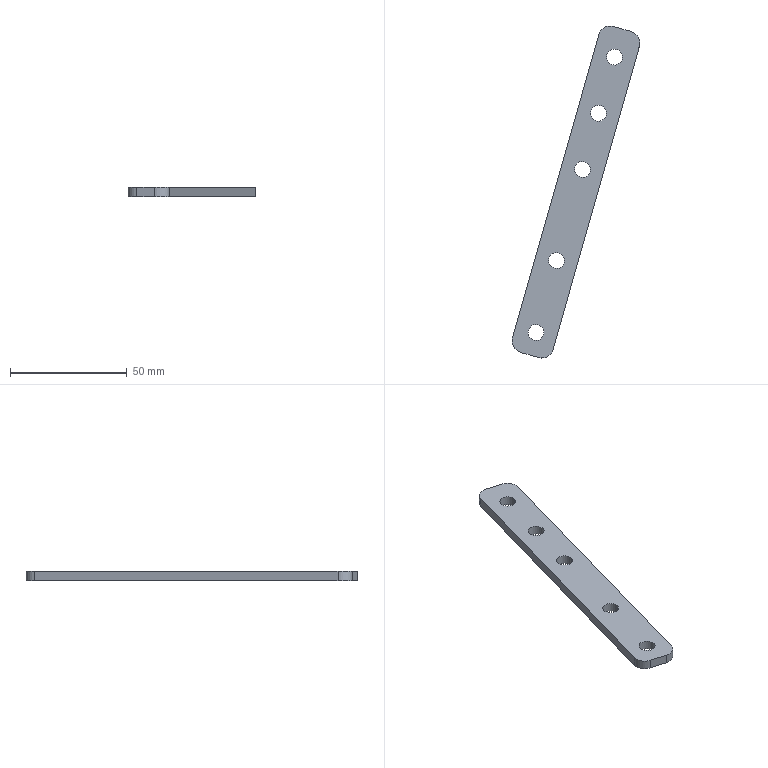Part | SolidWorks | features BaseBody 1 | 1 solid | 20 faces | box 54.655 x 142.032 x 4 mm | volume 9628 mm3 | cylinder 14 | plane 6 | commonest cylinder face diameters 6.8 x10 10 x4
STEP:
#1=CARTESIAN_POINT('',(427.437,245.838,55.5));
#2=VERTEX_POINT('',#1);
#3=CARTESIAN_POINT('',(420.897,247.7,55.5));
#4=VERTEX_POINT('',#3);
#5=CARTESIAN_POINT('',(424.167,246.769,55.5));
#6=DIRECTION('',(0.,0.,1.));
#7=DIRECTION('',(-0.9618,0.2738,0.));
#8=AXIS2_PLACEMENT_3D('',#5,#6,#7);
#9=CIRCLE('',#8,3.4);
#10=EDGE_CURVE('',#2,#4,#9,.T.);
#11=ORIENTED_EDGE('',*,*,#10,.F.);
#12=CARTESIAN_POINT('',(427.437,245.838,59.5));
#13=VERTEX_POINT('',#12);
#14=CARTESIAN_POINT('',(427.437,245.838,59.5));
#15=DIRECTION('',(0.,0.,1.));
#16=VECTOR('',#15,1000.);
#17=LINE('',#14,#16);
#18=EDGE_CURVE('',#2,#13,#17,.T.);
#19=ORIENTED_EDGE('',*,*,#18,.T.);
#20=CARTESIAN_POINT('',(420.897,247.7,59.5));
#21=VERTEX_POINT('',#20);
#22=CARTESIAN_POINT('',(424.167,246.769,59.5));
#23=DIRECTION('',(0.,0.,1.));
#24=DIRECTION('',(-0.9618,0.2738,0.));
#25=AXIS2_PLACEMENT_3D('',#22,#23,#24);
#26=CIRCLE('',#25,3.4);
#27=EDGE_CURVE('',#13,#21,#26,.T.);
#28=ORIENTED_EDGE('',*,*,#27,.T.);
#29=CARTESIAN_POINT('',(420.897,247.7,59.5));
#30=DIRECTION('',(0.,0.,1.));
#31=VECTOR('',#30,1000.);
#32=LINE('',#29,#31);
#33=EDGE_CURVE('',#4,#21,#32,.T.);
#34=ORIENTED_EDGE('',*,*,#33,.F.);
#35=EDGE_LOOP('',(#11,#19,#28,#34));
#36=FACE_OUTER_BOUND('',#35,.T.);
#37=CARTESIAN_POINT('',(424.167,246.769,59.5));
#38=DIRECTION('',(0.,0.,1.));
#39=DIRECTION('',(-0.9618,0.2738,0.));
#40=AXIS2_PLACEMENT_3D('',#37,#38,#39);
#41=CYLINDRICAL_SURFACE('',#40,3.4);
#42=ADVANCED_FACE('',(#36),#41,.F.);
#43=CARTESIAN_POINT('',(420.593,221.793,55.5));
#44=VERTEX_POINT('',#43);
#45=CARTESIAN_POINT('',(414.053,223.655,55.5));
#46=VERTEX_POINT('',#45);
#47=CARTESIAN_POINT('',(417.323,222.724,55.5));
#48=DIRECTION('',(0.,0.,1.));
#49=DIRECTION('',(-0.9618,0.2738,0.));
#50=AXIS2_PLACEMENT_3D('',#47,#48,#49);
#51=CIRCLE('',#50,3.4);
#52=EDGE_CURVE('',#44,#46,#51,.T.);
#53=ORIENTED_EDGE('',*,*,#52,.F.);
#54=CARTESIAN_POINT('',(420.593,221.793,59.5));
#55=VERTEX_POINT('',#54);
#56=CARTESIAN_POINT('',(420.593,221.793,59.5));
#57=DIRECTION('',(0.,0.,1.));
#58=VECTOR('',#57,1000.);
#59=LINE('',#56,#58);
#60=EDGE_CURVE('',#44,#55,#59,.T.);
#61=ORIENTED_EDGE('',*,*,#60,.T.);
#62=CARTESIAN_POINT('',(414.053,223.655,59.5));
#63=VERTEX_POINT('',#62);
#64=CARTESIAN_POINT('',(417.323,222.724,59.5));
#65=DIRECTION('',(0.,0.,1.));
#66=DIRECTION('',(-0.9618,0.2738,0.));
#67=AXIS2_PLACEMENT_3D('',#64,#65,#66);
#68=CIRCLE('',#67,3.4);
#69=EDGE_CURVE('',#55,#63,#68,.T.);
#70=ORIENTED_EDGE('',*,*,#69,.T.);
#71=CARTESIAN_POINT('',(414.053,223.655,59.5));
#72=DIRECTION('',(0.,0.,1.));
#73=VECTOR('',#72,1000.);
#74=LINE('',#71,#73);
#75=EDGE_CURVE('',#46,#63,#74,.T.);
#76=ORIENTED_EDGE('',*,*,#75,.F.);
#77=EDGE_LOOP('',(#53,#61,#70,#76));
#78=FACE_OUTER_BOUND('',#77,.T.);
#79=CARTESIAN_POINT('',(417.323,222.724,59.5));
#80=DIRECTION('',(0.,0.,1.));
#81=DIRECTION('',(-0.9618,0.2738,0.));
#82=AXIS2_PLACEMENT_3D('',#79,#80,#81);
#83=CYLINDRICAL_SURFACE('',#82,3.4);
#84=ADVANCED_FACE('',(#78),#83,.F.);
#85=CARTESIAN_POINT('',(413.748,197.748,55.5));
#86=VERTEX_POINT('',#85);
#87=CARTESIAN_POINT('',(407.208,199.61,55.5));
#88=VERTEX_POINT('',#87);
#89=CARTESIAN_POINT('',(410.478,198.679,55.5));
#90=DIRECTION('',(0.,0.,1.));
#91=DIRECTION('',(-0.9618,0.2738,0.));
#92=AXIS2_PLACEMENT_3D('',#89,#90,#91);
#93=CIRCLE('',#92,3.4);
#94=EDGE_CURVE('',#86,#88,#93,.T.);
#95=ORIENTED_EDGE('',*,*,#94,.F.);
#96=CARTESIAN_POINT('',(413.748,197.748,59.5));
#97=VERTEX_POINT('',#96);
#98=CARTESIAN_POINT('',(413.748,197.748,59.5));
#99=DIRECTION('',(0.,0.,1.));
#100=VECTOR('',#99,1000.);
#101=LINE('',#98,#100);
#102=EDGE_CURVE('',#86,#97,#101,.T.);
#103=ORIENTED_EDGE('',*,*,#102,.T.);
#104=CARTESIAN_POINT('',(407.208,199.61,59.5));
#105=VERTEX_POINT('',#104);
#106=CARTESIAN_POINT('',(410.478,198.679,59.5));
#107=DIRECTION('',(0.,0.,1.));
#108=DIRECTION('',(-0.9618,0.2738,0.));
#109=AXIS2_PLACEMENT_3D('',#106,#107,#108);
#110=CIRCLE('',#109,3.4);
#111=EDGE_CURVE('',#97,#105,#110,.T.);
#112=ORIENTED_EDGE('',*,*,#111,.T.);
#113=CARTESIAN_POINT('',(407.208,199.61,59.5));
#114=DIRECTION('',(0.,0.,1.));
#115=VECTOR('',#114,1000.);
#116=LINE('',#113,#115);
#117=EDGE_CURVE('',#88,#105,#116,.T.);
#118=ORIENTED_EDGE('',*,*,#117,.F.);
#119=EDGE_LOOP('',(#95,#103,#112,#118));
#120=FACE_OUTER_BOUND('',#119,.T.);
#121=CARTESIAN_POINT('',(410.478,198.679,59.5));
#122=DIRECTION('',(0.,0.,1.));
#123=DIRECTION('',(-0.9618,0.2738,0.));
#124=AXIS2_PLACEMENT_3D('',#121,#122,#123);
#125=CYLINDRICAL_SURFACE('',#124,3.4);
#126=ADVANCED_FACE('',(#120),#125,.F.);
#127=CARTESIAN_POINT('',(402.66,158.796,59.5));
#128=VERTEX_POINT('',#127);
#129=CARTESIAN_POINT('',(396.12,160.657,59.5));
#130=VERTEX_POINT('',#129);
#131=CARTESIAN_POINT('',(399.39,159.727,59.5));
#132=DIRECTION('',(0.,0.,1.));
#133=DIRECTION('',(-0.9618,0.2738,0.));
#134=AXIS2_PLACEMENT_3D('',#131,#132,#133);
#135=CIRCLE('',#134,3.4);
#136=EDGE_CURVE('',#128,#130,#135,.T.);
#137=ORIENTED_EDGE('',*,*,#136,.T.);
#138=CARTESIAN_POINT('',(396.12,160.657,55.5));
#139=VERTEX_POINT('',#138);
#140=CARTESIAN_POINT('',(396.12,160.657,59.5));
#141=DIRECTION('',(0.,0.,-1.));
#142=VECTOR('',#141,1000.);
#143=LINE('',#140,#142);
#144=EDGE_CURVE('',#130,#139,#143,.T.);
#145=ORIENTED_EDGE('',*,*,#144,.T.);
#146=CARTESIAN_POINT('',(402.66,158.796,55.5));
#147=VERTEX_POINT('',#146);
#148=CARTESIAN_POINT('',(399.39,159.727,55.5));
#149=DIRECTION('',(0.,0.,1.));
#150=DIRECTION('',(-0.9618,0.2738,0.));
#151=AXIS2_PLACEMENT_3D('',#148,#149,#150);
#152=CIRCLE('',#151,3.4);
#153=EDGE_CURVE('',#147,#139,#152,.T.);
#154=ORIENTED_EDGE('',*,*,#153,.F.);
#155=CARTESIAN_POINT('',(402.66,158.796,59.5));
#156=DIRECTION('',(0.,0.,-1.));
#157=VECTOR('',#156,1000.);
#158=LINE('',#155,#157);
#159=EDGE_CURVE('',#128,#147,#158,.T.);
#160=ORIENTED_EDGE('',*,*,#159,.F.);
#161=EDGE_LOOP('',(#137,#145,#154,#160));
#162=FACE_OUTER_BOUND('',#161,.T.);
#163=CARTESIAN_POINT('',(399.39,159.727,59.5));
#164=DIRECTION('',(0.,0.,-1.));
#165=DIRECTION('',(0.9618,-0.2738,0.));
#166=AXIS2_PLACEMENT_3D('',#163,#164,#165);
#167=CYLINDRICAL_SURFACE('',#166,3.4);
#168=ADVANCED_FACE('',(#162),#167,.F.);
#169=CARTESIAN_POINT('',(393.899,128.018,59.5));
#170=VERTEX_POINT('',#169);
#171=CARTESIAN_POINT('',(387.359,129.88,59.5));
#172=VERTEX_POINT('',#171);
#173=CARTESIAN_POINT('',(390.629,128.949,59.5));
#174=DIRECTION('',(0.,0.,1.));
#175=DIRECTION('',(-0.9618,0.2738,0.));
#176=AXIS2_PLACEMENT_3D('',#173,#174,#175);
#177=CIRCLE('',#176,3.4);
#178=EDGE_CURVE('',#170,#172,#177,.T.);
#179=ORIENTED_EDGE('',*,*,#178,.T.);
#180=CARTESIAN_POINT('',(387.359,129.88,55.5));
#181=VERTEX_POINT('',#180);
#182=CARTESIAN_POINT('',(387.359,129.88,59.5));
#183=DIRECTION('',(0.,0.,-1.));
#184=VECTOR('',#183,1000.);
#185=LINE('',#182,#184);
#186=EDGE_CURVE('',#172,#181,#185,.T.);
#187=ORIENTED_EDGE('',*,*,#186,.T.);
#188=CARTESIAN_POINT('',(393.899,128.018,55.5));
#189=VERTEX_POINT('',#188);
#190=CARTESIAN_POINT('',(390.629,128.949,55.5));
#191=DIRECTION('',(0.,0.,1.));
#192=DIRECTION('',(-0.9618,0.2738,0.));
#193=AXIS2_PLACEMENT_3D('',#190,#191,#192);
#194=CIRCLE('',#193,3.4);
#195=EDGE_CURVE('',#189,#181,#194,.T.);
#196=ORIENTED_EDGE('',*,*,#195,.F.);
#197=CARTESIAN_POINT('',(393.899,128.018,59.5));
#198=DIRECTION('',(0.,0.,-1.));
#199=VECTOR('',#198,1000.);
#200=LINE('',#197,#199);
#201=EDGE_CURVE('',#170,#189,#200,.T.);
#202=ORIENTED_EDGE('',*,*,#201,.F.);
#203=EDGE_LOOP('',(#179,#187,#196,#202));
#204=FACE_OUTER_BOUND('',#203,.T.);
#205=CARTESIAN_POINT('',(390.629,128.949,59.5));
#206=DIRECTION('',(0.,0.,-1.));
#207=DIRECTION('',(0.9618,-0.2738,0.));
#208=AXIS2_PLACEMENT_3D('',#205,#206,#207);
#209=CYLINDRICAL_SURFACE('',#208,3.4);
#210=ADVANCED_FACE('',(#204),#209,.F.);
#211=CARTESIAN_POINT('',(424.167,246.769,59.5));
#212=DIRECTION('',(0.,0.,1.));
#213=DIRECTION('',(-0.9618,0.2738,0.));
#214=AXIS2_PLACEMENT_3D('',#211,#212,#213);
#215=CIRCLE('',#214,3.4);
#216=EDGE_CURVE('',#21,#13,#215,.T.);
#217=ORIENTED_EDGE('',*,*,#216,.F.);
#218=ORIENTED_EDGE('',*,*,#27,.F.);
#219=EDGE_LOOP('',(#217,#218));
#220=FACE_BOUND('',#219,.T.);
#221=CARTESIAN_POINT('',(417.323,222.724,59.5));
#222=DIRECTION('',(0.,0.,1.));
#223=DIRECTION('',(-0.9618,0.2738,0.));
#224=AXIS2_PLACEMENT_3D('',#221,#222,#223);
#225=CIRCLE('',#224,3.4);
#226=EDGE_CURVE('',#63,#55,#225,.T.);
#227=ORIENTED_EDGE('',*,*,#226,.F.);
#228=ORIENTED_EDGE('',*,*,#69,.F.);
#229=EDGE_LOOP('',(#227,#228));
#230=FACE_BOUND('',#229,.T.);
#231=CARTESIAN_POINT('',(410.478,198.679,59.5));
#232=DIRECTION('',(0.,0.,1.));
#233=DIRECTION('',(-0.9618,0.2738,0.));
#234=AXIS2_PLACEMENT_3D('',#231,#232,#233);
#235=CIRCLE('',#234,3.4);
#236=EDGE_CURVE('',#105,#97,#235,.T.);
#237=ORIENTED_EDGE('',*,*,#236,.F.);
#238=ORIENTED_EDGE('',*,*,#111,.F.);
#239=EDGE_LOOP('',(#237,#238));
#240=FACE_BOUND('',#239,.T.);
#241=ORIENTED_EDGE('',*,*,#178,.F.);
#242=CARTESIAN_POINT('',(390.629,128.949,59.5));
#243=DIRECTION('',(0.,0.,1.));
#244=DIRECTION('',(-0.9618,0.2738,0.));
#245=AXIS2_PLACEMENT_3D('',#242,#243,#244);
#246=CIRCLE('',#245,3.4);
#247=EDGE_CURVE('',#172,#170,#246,.T.);
#248=ORIENTED_EDGE('',*,*,#247,.F.);
#249=EDGE_LOOP('',(#241,#248));
#250=FACE_BOUND('',#249,.T.);
#251=CARTESIAN_POINT('',(417.565,256.446,59.5));
#252=VERTEX_POINT('',#251);
#253=CARTESIAN_POINT('',(380.604,126.604,59.5));
#254=VERTEX_POINT('',#253);
#255=CARTESIAN_POINT('',(379.235,121.795,59.5));
#256=DIRECTION('',(-0.2738,-0.9618,0.));
#257=VECTOR('',#256,1000.);
#258=LINE('',#255,#257);
#259=EDGE_CURVE('',#252,#254,#258,.T.);
#260=ORIENTED_EDGE('',*,*,#259,.T.);
#261=CARTESIAN_POINT('',(384.044,120.426,59.5));
#262=VERTEX_POINT('',#261);
#263=CARTESIAN_POINT('',(385.413,125.235,59.5));
#264=DIRECTION('',(0.,0.,1.));
#265=DIRECTION('',(-0.9618,0.2738,0.));
#266=AXIS2_PLACEMENT_3D('',#263,#264,#265);
#267=CIRCLE('',#266,5.);
#268=EDGE_CURVE('',#254,#262,#267,.T.);
#269=ORIENTED_EDGE('',*,*,#268,.T.);
#270=CARTESIAN_POINT('',(391.738,118.236,59.5));
#271=VERTEX_POINT('',#270);
#272=CARTESIAN_POINT('',(396.547,116.867,59.5));
#273=DIRECTION('',(0.9618,-0.2738,0.));
#274=VECTOR('',#273,1000.);
#275=LINE('',#272,#274);
#276=EDGE_CURVE('',#262,#271,#275,.T.);
#277=ORIENTED_EDGE('',*,*,#276,.T.);
#278=CARTESIAN_POINT('',(397.916,121.676,59.5));
#279=VERTEX_POINT('',#278);
#280=CARTESIAN_POINT('',(393.107,123.045,59.5));
#281=DIRECTION('',(0.,0.,1.));
#282=DIRECTION('',(-0.9618,0.2738,0.));
#283=AXIS2_PLACEMENT_3D('',#280,#281,#282);
#284=CIRCLE('',#283,5.);
#285=EDGE_CURVE('',#271,#279,#284,.T.);
#286=ORIENTED_EDGE('',*,*,#285,.T.);
#287=CARTESIAN_POINT('',(434.877,251.518,59.5));
#288=VERTEX_POINT('',#287);
#289=CARTESIAN_POINT('',(396.547,116.867,59.5));
#290=DIRECTION('',(0.2738,0.9618,0.));
#291=VECTOR('',#290,1000.);
#292=LINE('',#289,#291);
#293=EDGE_CURVE('',#279,#288,#292,.T.);
#294=ORIENTED_EDGE('',*,*,#293,.T.);
#295=CARTESIAN_POINT('',(431.437,257.696,59.5));
#296=VERTEX_POINT('',#295);
#297=CARTESIAN_POINT('',(430.068,252.887,59.5));
#298=DIRECTION('',(0.,0.,1.));
#299=DIRECTION('',(-0.9618,0.2738,0.));
#300=AXIS2_PLACEMENT_3D('',#297,#298,#299);
#301=CIRCLE('',#300,5.);
#302=EDGE_CURVE('',#288,#296,#301,.T.);
#303=ORIENTED_EDGE('',*,*,#302,.T.);
#304=CARTESIAN_POINT('',(423.742,259.886,59.5));
#305=VERTEX_POINT('',#304);
#306=CARTESIAN_POINT('',(436.246,256.327,59.5));
#307=DIRECTION('',(-0.9618,0.2738,0.));
#308=VECTOR('',#307,1000.);
#309=LINE('',#306,#308);
#310=EDGE_CURVE('',#296,#305,#309,.T.);
#311=ORIENTED_EDGE('',*,*,#310,.T.);
#312=CARTESIAN_POINT('',(422.373,255.077,59.5));
#313=DIRECTION('',(0.,0.,1.));
#314=DIRECTION('',(-0.9618,0.2738,0.));
#315=AXIS2_PLACEMENT_3D('',#312,#313,#314);
#316=CIRCLE('',#315,5.);
#317=EDGE_CURVE('',#305,#252,#316,.T.);
#318=ORIENTED_EDGE('',*,*,#317,.T.);
#319=EDGE_LOOP('',(#260,#269,#277,#286,#294,#303,#311,#318));
#320=FACE_OUTER_BOUND('',#319,.T.);
#321=ORIENTED_EDGE('',*,*,#136,.F.);
#322=CARTESIAN_POINT('',(399.39,159.727,59.5));
#323=DIRECTION('',(0.,0.,1.));
#324=DIRECTION('',(-0.9618,0.2738,0.));
#325=AXIS2_PLACEMENT_3D('',#322,#323,#324);
#326=CIRCLE('',#325,3.4);
#327=EDGE_CURVE('',#130,#128,#326,.T.);
#328=ORIENTED_EDGE('',*,*,#327,.F.);
#329=EDGE_LOOP('',(#321,#328));
#330=FACE_BOUND('',#329,.T.);
#331=CARTESIAN_POINT('',(436.246,256.327,59.5));
#332=DIRECTION('',(0.,0.,1.));
#333=DIRECTION('',(-0.9618,0.2738,0.));
#334=AXIS2_PLACEMENT_3D('',#331,#332,#333);
#335=PLANE('',#334);
#336=ADVANCED_FACE('',(#220,#230,#240,#250,#320,#330),#335,.T.);
#337=CARTESIAN_POINT('',(424.167,246.769,55.5));
#338=DIRECTION('',(0.,0.,1.));
#339=DIRECTION('',(-0.9618,0.2738,0.));
#340=AXIS2_PLACEMENT_3D('',#337,#338,#339);
#341=CIRCLE('',#340,3.4);
#342=EDGE_CURVE('',#4,#2,#341,.T.);
#343=ORIENTED_EDGE('',*,*,#342,.T.);
#344=ORIENTED_EDGE('',*,*,#10,.T.);
#345=EDGE_LOOP('',(#343,#344));
#346=FACE_BOUND('',#345,.T.);
#347=CARTESIAN_POINT('',(417.323,222.724,55.5));
#348=DIRECTION('',(0.,0.,1.));
#349=DIRECTION('',(-0.9618,0.2738,0.));
#350=AXIS2_PLACEMENT_3D('',#347,#348,#349);
#351=CIRCLE('',#350,3.4);
#352=EDGE_CURVE('',#46,#44,#351,.T.);
#353=ORIENTED_EDGE('',*,*,#352,.T.);
#354=ORIENTED_EDGE('',*,*,#52,.T.);
#355=EDGE_LOOP('',(#353,#354));
#356=FACE_BOUND('',#355,.T.);
#357=CARTESIAN_POINT('',(410.478,198.679,55.5));
#358=DIRECTION('',(0.,0.,1.));
#359=DIRECTION('',(-0.9618,0.2738,0.));
#360=AXIS2_PLACEMENT_3D('',#357,#358,#359);
#361=CIRCLE('',#360,3.4);
#362=EDGE_CURVE('',#88,#86,#361,.T.);
#363=ORIENTED_EDGE('',*,*,#362,.T.);
#364=ORIENTED_EDGE('',*,*,#94,.T.);
#365=EDGE_LOOP('',(#363,#364));
#366=FACE_BOUND('',#365,.T.);
#367=ORIENTED_EDGE('',*,*,#195,.T.);
#368=CARTESIAN_POINT('',(390.629,128.949,55.5));
#369=DIRECTION('',(0.,0.,1.));
#370=DIRECTION('',(-0.9618,0.2738,0.));
#371=AXIS2_PLACEMENT_3D('',#368,#369,#370);
#372=CIRCLE('',#371,3.4);
#373=EDGE_CURVE('',#181,#189,#372,.T.);
#374=ORIENTED_EDGE('',*,*,#373,.T.);
#375=EDGE_LOOP('',(#367,#374));
#376=FACE_BOUND('',#375,.T.);
#377=CARTESIAN_POINT('',(384.044,120.426,55.5));
#378=VERTEX_POINT('',#377);
#379=CARTESIAN_POINT('',(391.738,118.236,55.5));
#380=VERTEX_POINT('',#379);
#381=CARTESIAN_POINT('',(396.547,116.867,55.5));
#382=DIRECTION('',(0.9618,-0.2738,0.));
#383=VECTOR('',#382,1000.);
#384=LINE('',#381,#383);
#385=EDGE_CURVE('',#378,#380,#384,.T.);
#386=ORIENTED_EDGE('',*,*,#385,.F.);
#387=CARTESIAN_POINT('',(380.604,126.604,55.5));
#388=VERTEX_POINT('',#387);
#389=CARTESIAN_POINT('',(385.413,125.235,55.5));
#390=DIRECTION('',(0.,0.,-1.));
#391=DIRECTION('',(-0.9618,0.2738,0.));
#392=AXIS2_PLACEMENT_3D('',#389,#390,#391);
#393=CIRCLE('',#392,5.);
#394=EDGE_CURVE('',#378,#388,#393,.T.);
#395=ORIENTED_EDGE('',*,*,#394,.T.);
#396=CARTESIAN_POINT('',(417.565,256.446,55.5));
#397=VERTEX_POINT('',#396);
#398=CARTESIAN_POINT('',(379.235,121.795,55.5));
#399=DIRECTION('',(-0.2738,-0.9618,0.));
#400=VECTOR('',#399,1000.);
#401=LINE('',#398,#400);
#402=EDGE_CURVE('',#397,#388,#401,.T.);
#403=ORIENTED_EDGE('',*,*,#402,.F.);
#404=CARTESIAN_POINT('',(423.742,259.886,55.5));
#405=VERTEX_POINT('',#404);
#406=CARTESIAN_POINT('',(422.373,255.077,55.5));
#407=DIRECTION('',(0.,0.,-1.));
#408=DIRECTION('',(-0.9618,0.2738,0.));
#409=AXIS2_PLACEMENT_3D('',#406,#407,#408);
#410=CIRCLE('',#409,5.);
#411=EDGE_CURVE('',#397,#405,#410,.T.);
#412=ORIENTED_EDGE('',*,*,#411,.T.);
#413=CARTESIAN_POINT('',(431.437,257.696,55.5));
#414=VERTEX_POINT('',#413);
#415=CARTESIAN_POINT('',(436.246,256.327,55.5));
#416=DIRECTION('',(-0.9618,0.2738,0.));
#417=VECTOR('',#416,1000.);
#418=LINE('',#415,#417);
#419=EDGE_CURVE('',#414,#405,#418,.T.);
#420=ORIENTED_EDGE('',*,*,#419,.F.);
#421=CARTESIAN_POINT('',(434.877,251.518,55.5));
#422=VERTEX_POINT('',#421);
#423=CARTESIAN_POINT('',(430.068,252.887,55.5));
#424=DIRECTION('',(0.,0.,-1.));
#425=DIRECTION('',(-0.9618,0.2738,0.));
#426=AXIS2_PLACEMENT_3D('',#423,#424,#425);
#427=CIRCLE('',#426,5.);
#428=EDGE_CURVE('',#414,#422,#427,.T.);
#429=ORIENTED_EDGE('',*,*,#428,.T.);
#430=CARTESIAN_POINT('',(397.916,121.676,55.5));
#431=VERTEX_POINT('',#430);
#432=CARTESIAN_POINT('',(396.547,116.867,55.5));
#433=DIRECTION('',(0.2738,0.9618,0.));
#434=VECTOR('',#433,1000.);
#435=LINE('',#432,#434);
#436=EDGE_CURVE('',#431,#422,#435,.T.);
#437=ORIENTED_EDGE('',*,*,#436,.F.);
#438=CARTESIAN_POINT('',(393.107,123.045,55.5));
#439=DIRECTION('',(0.,0.,-1.));
#440=DIRECTION('',(-0.9618,0.2738,0.));
#441=AXIS2_PLACEMENT_3D('',#438,#439,#440);
#442=CIRCLE('',#441,5.);
#443=EDGE_CURVE('',#431,#380,#442,.T.);
#444=ORIENTED_EDGE('',*,*,#443,.T.);
#445=EDGE_LOOP('',(#386,#395,#403,#412,#420,#429,#437,#444));
#446=FACE_OUTER_BOUND('',#445,.T.);
#447=ORIENTED_EDGE('',*,*,#153,.T.);
#448=CARTESIAN_POINT('',(399.39,159.727,55.5));
#449=DIRECTION('',(0.,0.,1.));
#450=DIRECTION('',(-0.9618,0.2738,0.));
#451=AXIS2_PLACEMENT_3D('',#448,#449,#450);
#452=CIRCLE('',#451,3.4);
#453=EDGE_CURVE('',#139,#147,#452,.T.);
#454=ORIENTED_EDGE('',*,*,#453,.T.);
#455=EDGE_LOOP('',(#447,#454));
#456=FACE_BOUND('',#455,.T.);
#457=CARTESIAN_POINT('',(436.246,256.327,55.5));
#458=DIRECTION('',(0.,0.,1.));
#459=DIRECTION('',(-0.9618,0.2738,0.));
#460=AXIS2_PLACEMENT_3D('',#457,#458,#459);
#461=PLANE('',#460);
#462=ADVANCED_FACE('',(#346,#356,#366,#376,#446,#456),#461,.F.);
#463=ORIENTED_EDGE('',*,*,#293,.F.);
#464=CARTESIAN_POINT('',(397.916,121.676,59.5));
#465=DIRECTION('',(0.,0.,-1.));
#466=VECTOR('',#465,1000.);
#467=LINE('',#464,#466);
#468=EDGE_CURVE('',#279,#431,#467,.T.);
#469=ORIENTED_EDGE('',*,*,#468,.T.);
#470=ORIENTED_EDGE('',*,*,#436,.T.);
#471=CARTESIAN_POINT('',(434.877,251.518,59.5));
#472=DIRECTION('',(0.,0.,1.));
#473=VECTOR('',#472,1000.);
#474=LINE('',#471,#473);
#475=EDGE_CURVE('',#422,#288,#474,.T.);
#476=ORIENTED_EDGE('',*,*,#475,.T.);
#477=EDGE_LOOP('',(#463,#469,#470,#476));
#478=FACE_OUTER_BOUND('',#477,.T.);
#479=CARTESIAN_POINT('',(396.547,116.867,59.5));
#480=DIRECTION('',(-0.9618,0.2738,0.));
#481=DIRECTION('',(-0.2738,-0.9618,0.));
#482=AXIS2_PLACEMENT_3D('',#479,#480,#481);
#483=PLANE('',#482);
#484=ADVANCED_FACE('',(#478),#483,.F.);
#485=ORIENTED_EDGE('',*,*,#419,.T.);
#486=CARTESIAN_POINT('',(423.742,259.886,59.5));
#487=DIRECTION('',(0.,0.,1.));
#488=VECTOR('',#487,1000.);
#489=LINE('',#486,#488);
#490=EDGE_CURVE('',#405,#305,#489,.T.);
#491=ORIENTED_EDGE('',*,*,#490,.T.);
#492=ORIENTED_EDGE('',*,*,#310,.F.);
#493=CARTESIAN_POINT('',(431.437,257.696,59.5));
#494=DIRECTION('',(0.,0.,-1.));
#495=VECTOR('',#494,1000.);
#496=LINE('',#493,#495);
#497=EDGE_CURVE('',#296,#414,#496,.T.);
#498=ORIENTED_EDGE('',*,*,#497,.T.);
#499=EDGE_LOOP('',(#485,#491,#492,#498));
#500=FACE_OUTER_BOUND('',#499,.T.);
#501=CARTESIAN_POINT('',(436.246,256.327,59.5));
#502=DIRECTION('',(-0.2738,-0.9618,0.));
#503=DIRECTION('',(0.9618,-0.2738,0.));
#504=AXIS2_PLACEMENT_3D('',#501,#502,#503);
#505=PLANE('',#504);
#506=ADVANCED_FACE('',(#500),#505,.F.);
#507=ORIENTED_EDGE('',*,*,#402,.T.);
#508=CARTESIAN_POINT('',(380.604,126.604,59.5));
#509=DIRECTION('',(0.,0.,1.));
#510=VECTOR('',#509,1000.);
#511=LINE('',#508,#510);
#512=EDGE_CURVE('',#388,#254,#511,.T.);
#513=ORIENTED_EDGE('',*,*,#512,.T.);
#514=ORIENTED_EDGE('',*,*,#259,.F.);
#515=CARTESIAN_POINT('',(417.565,256.446,59.5));
#516=DIRECTION('',(0.,0.,-1.));
#517=VECTOR('',#516,1000.);
#518=LINE('',#515,#517);
#519=EDGE_CURVE('',#252,#397,#518,.T.);
#520=ORIENTED_EDGE('',*,*,#519,.T.);
#521=EDGE_LOOP('',(#507,#513,#514,#520));
#522=FACE_OUTER_BOUND('',#521,.T.);
#523=CARTESIAN_POINT('',(379.235,121.795,59.5));
#524=DIRECTION('',(0.9618,-0.2738,0.));
#525=DIRECTION('',(0.2738,0.9618,0.));
#526=AXIS2_PLACEMENT_3D('',#523,#524,#525);
#527=PLANE('',#526);
#528=ADVANCED_FACE('',(#522),#527,.F.);
#529=ORIENTED_EDGE('',*,*,#276,.F.);
#530=CARTESIAN_POINT('',(384.044,120.426,59.5));
#531=DIRECTION('',(0.,0.,-1.));
#532=VECTOR('',#531,1000.);
#533=LINE('',#530,#532);
#534=EDGE_CURVE('',#262,#378,#533,.T.);
#535=ORIENTED_EDGE('',*,*,#534,.T.);
#536=ORIENTED_EDGE('',*,*,#385,.T.);
#537=CARTESIAN_POINT('',(391.738,118.236,59.5));
#538=DIRECTION('',(0.,0.,1.));
#539=VECTOR('',#538,1000.);
#540=LINE('',#537,#539);
#541=EDGE_CURVE('',#380,#271,#540,.T.);
#542=ORIENTED_EDGE('',*,*,#541,.T.);
#543=EDGE_LOOP('',(#529,#535,#536,#542));
#544=FACE_OUTER_BOUND('',#543,.T.);
#545=CARTESIAN_POINT('',(396.547,116.867,59.5));
#546=DIRECTION('',(0.2738,0.9618,0.));
#547=DIRECTION('',(-0.9618,0.2738,0.));
#548=AXIS2_PLACEMENT_3D('',#545,#546,#547);
#549=PLANE('',#548);
#550=ADVANCED_FACE('',(#544),#549,.F.);
#551=ORIENTED_EDGE('',*,*,#186,.F.);
#552=ORIENTED_EDGE('',*,*,#247,.T.);
#553=ORIENTED_EDGE('',*,*,#201,.T.);
#554=ORIENTED_EDGE('',*,*,#373,.F.);
#555=EDGE_LOOP('',(#551,#552,#553,#554));
#556=FACE_OUTER_BOUND('',#555,.T.);
#557=CARTESIAN_POINT('',(390.629,128.949,59.5));
#558=DIRECTION('',(0.,0.,-1.));
#559=DIRECTION('',(0.9618,-0.2738,0.));
#560=AXIS2_PLACEMENT_3D('',#557,#558,#559);
#561=CYLINDRICAL_SURFACE('',#560,3.4);
#562=ADVANCED_FACE('',(#556),#561,.F.);
#563=ORIENTED_EDGE('',*,*,#144,.F.);
#564=ORIENTED_EDGE('',*,*,#327,.T.);
#565=ORIENTED_EDGE('',*,*,#159,.T.);
#566=ORIENTED_EDGE('',*,*,#453,.F.);
#567=EDGE_LOOP('',(#563,#564,#565,#566));
#568=FACE_OUTER_BOUND('',#567,.T.);
#569=CARTESIAN_POINT('',(399.39,159.727,59.5));
#570=DIRECTION('',(0.,0.,-1.));
#571=DIRECTION('',(0.9618,-0.2738,0.));
#572=AXIS2_PLACEMENT_3D('',#569,#570,#571);
#573=CYLINDRICAL_SURFACE('',#572,3.4);
#574=ADVANCED_FACE('',(#568),#573,.F.);
#575=ORIENTED_EDGE('',*,*,#102,.F.);
#576=ORIENTED_EDGE('',*,*,#362,.F.);
#577=ORIENTED_EDGE('',*,*,#117,.T.);
#578=ORIENTED_EDGE('',*,*,#236,.T.);
#579=EDGE_LOOP('',(#575,#576,#577,#578));
#580=FACE_OUTER_BOUND('',#579,.T.);
#581=CARTESIAN_POINT('',(410.478,198.679,59.5));
#582=DIRECTION('',(0.,0.,1.));
#583=DIRECTION('',(-0.9618,0.2738,0.));
#584=AXIS2_PLACEMENT_3D('',#581,#582,#583);
#585=CYLINDRICAL_SURFACE('',#584,3.4);
#586=ADVANCED_FACE('',(#580),#585,.F.);
#587=ORIENTED_EDGE('',*,*,#60,.F.);
#588=ORIENTED_EDGE('',*,*,#352,.F.);
#589=ORIENTED_EDGE('',*,*,#75,.T.);
#590=ORIENTED_EDGE('',*,*,#226,.T.);
#591=EDGE_LOOP('',(#587,#588,#589,#590));
#592=FACE_OUTER_BOUND('',#591,.T.);
#593=CARTESIAN_POINT('',(417.323,222.724,59.5));
#594=DIRECTION('',(0.,0.,1.));
#595=DIRECTION('',(-0.9618,0.2738,0.));
#596=AXIS2_PLACEMENT_3D('',#593,#594,#595);
#597=CYLINDRICAL_SURFACE('',#596,3.4);
#598=ADVANCED_FACE('',(#592),#597,.F.);
#599=ORIENTED_EDGE('',*,*,#18,.F.);
#600=ORIENTED_EDGE('',*,*,#342,.F.);
#601=ORIENTED_EDGE('',*,*,#33,.T.);
#602=ORIENTED_EDGE('',*,*,#216,.T.);
#603=EDGE_LOOP('',(#599,#600,#601,#602));
#604=FACE_OUTER_BOUND('',#603,.T.);
#605=CARTESIAN_POINT('',(424.167,246.769,59.5));
#606=DIRECTION('',(0.,0.,1.));
#607=DIRECTION('',(-0.9618,0.2738,0.));
#608=AXIS2_PLACEMENT_3D('',#605,#606,#607);
#609=CYLINDRICAL_SURFACE('',#608,3.4);
#610=ADVANCED_FACE('',(#604),#609,.F.);
#611=ORIENTED_EDGE('',*,*,#268,.F.);
#612=ORIENTED_EDGE('',*,*,#512,.F.);
#613=ORIENTED_EDGE('',*,*,#394,.F.);
#614=ORIENTED_EDGE('',*,*,#534,.F.);
#615=EDGE_LOOP('',(#611,#612,#613,#614));
#616=FACE_OUTER_BOUND('',#615,.T.);
#617=CARTESIAN_POINT('',(385.413,125.235,59.5));
#618=DIRECTION('',(0.,0.,-1.));
#619=DIRECTION('',(0.9618,-0.2738,0.));
#620=AXIS2_PLACEMENT_3D('',#617,#618,#619);
#621=CYLINDRICAL_SURFACE('',#620,5.);
#622=ADVANCED_FACE('',(#616),#621,.T.);
#623=ORIENTED_EDGE('',*,*,#285,.F.);
#624=ORIENTED_EDGE('',*,*,#541,.F.);
#625=ORIENTED_EDGE('',*,*,#443,.F.);
#626=ORIENTED_EDGE('',*,*,#468,.F.);
#627=EDGE_LOOP('',(#623,#624,#625,#626));
#628=FACE_OUTER_BOUND('',#627,.T.);
#629=CARTESIAN_POINT('',(393.107,123.045,59.5));
#630=DIRECTION('',(0.,0.,-1.));
#631=DIRECTION('',(0.9618,-0.2738,0.));
#632=AXIS2_PLACEMENT_3D('',#629,#630,#631);
#633=CYLINDRICAL_SURFACE('',#632,5.);
#634=ADVANCED_FACE('',(#628),#633,.T.);
#635=ORIENTED_EDGE('',*,*,#317,.F.);
#636=ORIENTED_EDGE('',*,*,#490,.F.);
#637=ORIENTED_EDGE('',*,*,#411,.F.);
#638=ORIENTED_EDGE('',*,*,#519,.F.);
#639=EDGE_LOOP('',(#635,#636,#637,#638));
#640=FACE_OUTER_BOUND('',#639,.T.);
#641=CARTESIAN_POINT('',(422.373,255.077,59.5));
#642=DIRECTION('',(0.,0.,-1.));
#643=DIRECTION('',(0.9618,-0.2738,0.));
#644=AXIS2_PLACEMENT_3D('',#641,#642,#643);
#645=CYLINDRICAL_SURFACE('',#644,5.);
#646=ADVANCED_FACE('',(#640),#645,.T.);
#647=ORIENTED_EDGE('',*,*,#302,.F.);
#648=ORIENTED_EDGE('',*,*,#475,.F.);
#649=ORIENTED_EDGE('',*,*,#428,.F.);
#650=ORIENTED_EDGE('',*,*,#497,.F.);
#651=EDGE_LOOP('',(#647,#648,#649,#650));
#652=FACE_OUTER_BOUND('',#651,.T.);
#653=CARTESIAN_POINT('',(430.068,252.887,59.5));
#654=DIRECTION('',(0.,0.,-1.));
#655=DIRECTION('',(0.9618,-0.2738,0.));
#656=AXIS2_PLACEMENT_3D('',#653,#654,#655);
#657=CYLINDRICAL_SURFACE('',#656,5.);
#658=ADVANCED_FACE('',(#652),#657,.T.);
#659=CLOSED_SHELL('',(#42,#84,#126,#168,#210,#336,#462,#484,#506,#528,#550,#562,#574,#586,#598,#610,#622,#634,#646,#658));
#660=MANIFOLD_SOLID_BREP('',#659);
#661=CARTESIAN_POINT('',(0.,0.,0.));
#662=DIRECTION('',(0.,0.,1.));
#663=DIRECTION('',(1.,0.,0.));
#664=AXIS2_PLACEMENT_3D('',#661,#662,#663);
#665=(LENGTH_UNIT()NAMED_UNIT(*)SI_UNIT(.MILLI.,.METRE.));
#666=UNCERTAINTY_MEASURE_WITH_UNIT(LENGTH_MEASURE(0.00001),#665,'','');
#667=(NAMED_UNIT(*)PLANE_ANGLE_UNIT()SI_UNIT($,.RADIAN.));
#668=(NAMED_UNIT(*)SI_UNIT($,.STERADIAN.)SOLID_ANGLE_UNIT());
#669=(GEOMETRIC_REPRESENTATION_CONTEXT(3)GLOBAL_UNCERTAINTY_ASSIGNED_CONTEXT((#666))GLOBAL_UNIT_ASSIGNED_CONTEXT((#665,#667,#668))REPRESENTATION_CONTEXT('',''));
#670=ADVANCED_BREP_SHAPE_REPRESENTATION('',(#660,#664),#669);